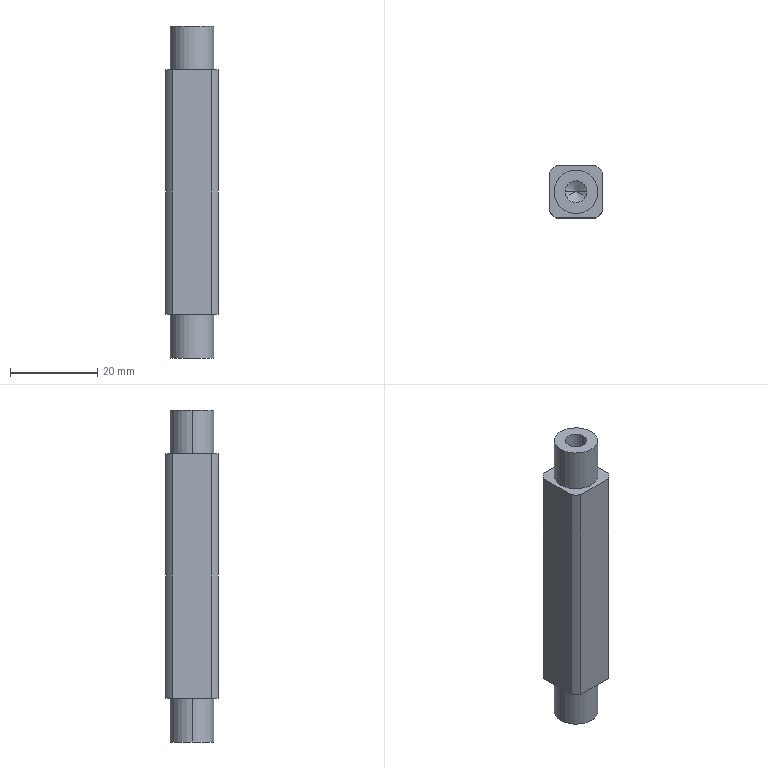Part | STEP file | Fixed shaft QY-1-07 | 1 solid | 20 faces | box 12 x 12 x 76 mm | volume 9102 mm3 | cylinder 10 | plane 8 | cone 2 | commonest cylinder face diameters 10 x4 15 x4 5 x2
STEP:
#1=CARTESIAN_POINT('',(0.,0.,0.));
#2=DIRECTION('',(0.,0.,1.));
#3=DIRECTION('',(1.,0.,0.));
#4=AXIS2_PLACEMENT_3D('',#1,#2,#3);
#5=CARTESIAN_POINT('',(2.5,0.,23.));
#6=VERTEX_POINT('',#5);
#7=CARTESIAN_POINT('',(2.5,0.,38.));
#8=VERTEX_POINT('',#7);
#9=CARTESIAN_POINT('',(2.5,0.,38.));
#10=DIRECTION('',(0.,0.,1.));
#11=VECTOR('',#10,1.);
#12=LINE('',#9,#11);
#13=CARTESIAN_POINT('',(0.,0.,38.));
#14=DIRECTION('',(0.,0.,1.));
#15=DIRECTION('',(1.,0.,0.));
#16=AXIS2_PLACEMENT_3D('',#13,#14,#15);
#17=CYLINDRICAL_SURFACE('',#16,2.5);
#18=CARTESIAN_POINT('',(6.283,0.));
#19=DIRECTION('',(0.,1.));
#20=VECTOR('',#19,1.);
#21=LINE('',#18,#20);
#22=(GEOMETRIC_REPRESENTATION_CONTEXT(2)PARAMETRIC_REPRESENTATION_CONTEXT()REPRESENTATION_CONTEXT('',''));
#23=DEFINITIONAL_REPRESENTATION('',(#21),#22);
#24=PCURVE('',#17,#23);
#25=CARTESIAN_POINT('',(0.,0.,38.));
#26=DIRECTION('',(0.,0.,1.));
#27=DIRECTION('',(1.,0.,0.));
#28=AXIS2_PLACEMENT_3D('',#25,#26,#27);
#29=CYLINDRICAL_SURFACE('',#28,2.5);
#30=CARTESIAN_POINT('',(0.,0.));
#31=DIRECTION('',(0.,1.));
#32=VECTOR('',#31,1.);
#33=LINE('',#30,#32);
#34=(GEOMETRIC_REPRESENTATION_CONTEXT(2)PARAMETRIC_REPRESENTATION_CONTEXT()REPRESENTATION_CONTEXT('',''));
#35=DEFINITIONAL_REPRESENTATION('',(#33),#34);
#36=PCURVE('',#29,#35);
#37=SURFACE_CURVE('',#12,(#24,#36),.PCURVE_S1.);
#38=EDGE_CURVE('',#6,#8,#37,.T.);
#39=ORIENTED_EDGE('',*,*,#38,.T.);
#40=CARTESIAN_POINT('',(-2.5,0.,38.));
#41=VERTEX_POINT('',#40);
#42=CARTESIAN_POINT('',(0.,0.,38.));
#43=DIRECTION('',(0.,0.,1.));
#44=DIRECTION('',(1.,0.,0.));
#45=AXIS2_PLACEMENT_3D('',#42,#43,#44);
#46=CIRCLE('',#45,2.5);
#47=CARTESIAN_POINT('',(0.,0.));
#48=DIRECTION('',(1.,0.));
#49=VECTOR('',#48,1.);
#50=LINE('',#47,#49);
#51=(GEOMETRIC_REPRESENTATION_CONTEXT(2)PARAMETRIC_REPRESENTATION_CONTEXT()REPRESENTATION_CONTEXT('',''));
#52=DEFINITIONAL_REPRESENTATION('',(#50),#51);
#53=PCURVE('',#17,#52);
#54=CARTESIAN_POINT('',(0.,0.,38.));
#55=DIRECTION('',(0.,0.,1.));
#56=DIRECTION('',(1.,0.,0.));
#57=AXIS2_PLACEMENT_3D('',#54,#55,#56);
#58=PLANE('',#57);
#59=CARTESIAN_POINT('',(0.,0.));
#60=DIRECTION('',(1.,0.));
#61=AXIS2_PLACEMENT_2D('',#59,#60);
#62=CIRCLE('',#61,2.5);
#63=(GEOMETRIC_REPRESENTATION_CONTEXT(2)PARAMETRIC_REPRESENTATION_CONTEXT()REPRESENTATION_CONTEXT('',''));
#64=DEFINITIONAL_REPRESENTATION('',(#62),#63);
#65=PCURVE('',#58,#64);
#66=SURFACE_CURVE('',#46,(#53,#65),.PCURVE_S1.);
#67=EDGE_CURVE('',#41,#8,#66,.T.);
#68=ORIENTED_EDGE('',*,*,#67,.F.);
#69=CARTESIAN_POINT('',(-2.5,0.,23.));
#70=VERTEX_POINT('',#69);
#71=CARTESIAN_POINT('',(-2.5,0.,38.));
#72=DIRECTION('',(0.,0.,1.));
#73=VECTOR('',#72,1.);
#74=LINE('',#71,#73);
#75=CARTESIAN_POINT('',(3.142,0.));
#76=DIRECTION('',(0.,1.));
#77=VECTOR('',#76,1.);
#78=LINE('',#75,#77);
#79=(GEOMETRIC_REPRESENTATION_CONTEXT(2)PARAMETRIC_REPRESENTATION_CONTEXT()REPRESENTATION_CONTEXT('',''));
#80=DEFINITIONAL_REPRESENTATION('',(#78),#79);
#81=PCURVE('',#17,#80);
#82=CARTESIAN_POINT('',(3.142,0.));
#83=DIRECTION('',(0.,1.));
#84=VECTOR('',#83,1.);
#85=LINE('',#82,#84);
#86=(GEOMETRIC_REPRESENTATION_CONTEXT(2)PARAMETRIC_REPRESENTATION_CONTEXT()REPRESENTATION_CONTEXT('',''));
#87=DEFINITIONAL_REPRESENTATION('',(#85),#86);
#88=PCURVE('',#29,#87);
#89=SURFACE_CURVE('',#74,(#81,#88),.PCURVE_S1.);
#90=EDGE_CURVE('',#70,#41,#89,.T.);
#91=ORIENTED_EDGE('',*,*,#90,.F.);
#92=CARTESIAN_POINT('',(0.,0.,23.));
#93=DIRECTION('',(0.,0.,1.));
#94=DIRECTION('',(1.,0.,0.));
#95=AXIS2_PLACEMENT_3D('',#92,#93,#94);
#96=CIRCLE('',#95,2.5);
#97=CARTESIAN_POINT('',(0.,-15.));
#98=DIRECTION('',(1.,0.));
#99=VECTOR('',#98,1.);
#100=LINE('',#97,#99);
#101=(GEOMETRIC_REPRESENTATION_CONTEXT(2)PARAMETRIC_REPRESENTATION_CONTEXT()REPRESENTATION_CONTEXT('',''));
#102=DEFINITIONAL_REPRESENTATION('',(#100),#101);
#103=PCURVE('',#17,#102);
#104=CARTESIAN_POINT('',(0.,0.,23.));
#105=DIRECTION('',(0.,0.,1.));
#106=DIRECTION('',(1.,0.,0.));
#107=AXIS2_PLACEMENT_3D('',#104,#105,#106);
#108=CONICAL_SURFACE('',#107,2.5,1.03);
#109=CARTESIAN_POINT('',(0.,0.));
#110=DIRECTION('',(1.,0.));
#111=VECTOR('',#110,1.);
#112=LINE('',#109,#111);
#113=(GEOMETRIC_REPRESENTATION_CONTEXT(2)PARAMETRIC_REPRESENTATION_CONTEXT()REPRESENTATION_CONTEXT('',''));
#114=DEFINITIONAL_REPRESENTATION('',(#112),#113);
#115=PCURVE('',#108,#114);
#116=SURFACE_CURVE('',#96,(#103,#115),.PCURVE_S1.);
#117=EDGE_CURVE('',#70,#6,#116,.T.);
#118=ORIENTED_EDGE('',*,*,#117,.T.);
#119=EDGE_LOOP('',(#39,#68,#91,#118));
#120=FACE_BOUND('',#119,.F.);
#121=ADVANCED_FACE('',(#120),#17,.F.);
#122=ORIENTED_EDGE('',*,*,#117,.F.);
#123=CARTESIAN_POINT('',(0.,0.,21.498));
#124=VERTEX_POINT('',#123);
#125=CARTESIAN_POINT('',(-2.5,0.,23.));
#126=DIRECTION('',(-0.8572,0.,0.515));
#127=VECTOR('',#126,1.);
#128=LINE('',#125,#127);
#129=CARTESIAN_POINT('',(3.142,0.));
#130=DIRECTION('',(0.,1.));
#131=VECTOR('',#130,1.);
#132=LINE('',#129,#131);
#133=(GEOMETRIC_REPRESENTATION_CONTEXT(2)PARAMETRIC_REPRESENTATION_CONTEXT()REPRESENTATION_CONTEXT('',''));
#134=DEFINITIONAL_REPRESENTATION('',(#132),#133);
#135=PCURVE('',#108,#134);
#136=CARTESIAN_POINT('',(0.,0.,23.));
#137=DIRECTION('',(0.,0.,1.));
#138=DIRECTION('',(1.,0.,0.));
#139=AXIS2_PLACEMENT_3D('',#136,#137,#138);
#140=CONICAL_SURFACE('',#139,2.5,1.03);
#141=CARTESIAN_POINT('',(3.142,0.));
#142=DIRECTION('',(0.,1.));
#143=VECTOR('',#142,1.);
#144=LINE('',#141,#143);
#145=(GEOMETRIC_REPRESENTATION_CONTEXT(2)PARAMETRIC_REPRESENTATION_CONTEXT()REPRESENTATION_CONTEXT('',''));
#146=DEFINITIONAL_REPRESENTATION('',(#144),#145);
#147=PCURVE('',#140,#146);
#148=SURFACE_CURVE('',#128,(#135,#147),.PCURVE_S1.);
#149=EDGE_CURVE('',#124,#70,#148,.T.);
#150=ORIENTED_EDGE('',*,*,#149,.F.);
#151=CARTESIAN_POINT('',(2.5,0.,23.));
#152=DIRECTION('',(0.8572,0.,0.515));
#153=VECTOR('',#152,1.);
#154=LINE('',#151,#153);
#155=CARTESIAN_POINT('',(6.283,0.));
#156=DIRECTION('',(0.,1.));
#157=VECTOR('',#156,1.);
#158=LINE('',#155,#157);
#159=(GEOMETRIC_REPRESENTATION_CONTEXT(2)PARAMETRIC_REPRESENTATION_CONTEXT()REPRESENTATION_CONTEXT('',''));
#160=DEFINITIONAL_REPRESENTATION('',(#158),#159);
#161=PCURVE('',#108,#160);
#162=CARTESIAN_POINT('',(0.,0.));
#163=DIRECTION('',(0.,1.));
#164=VECTOR('',#163,1.);
#165=LINE('',#162,#164);
#166=(GEOMETRIC_REPRESENTATION_CONTEXT(2)PARAMETRIC_REPRESENTATION_CONTEXT()REPRESENTATION_CONTEXT('',''));
#167=DEFINITIONAL_REPRESENTATION('',(#165),#166);
#168=PCURVE('',#140,#167);
#169=SURFACE_CURVE('',#154,(#161,#168),.PCURVE_S1.);
#170=EDGE_CURVE('',#124,#6,#169,.T.);
#171=ORIENTED_EDGE('',*,*,#170,.T.);
#172=EDGE_LOOP('',(#122,#150,#171));
#173=FACE_BOUND('',#172,.F.);
#174=ADVANCED_FACE('',(#173),#108,.F.);
#175=CARTESIAN_POINT('',(5.,0.,-38.));
#176=VERTEX_POINT('',#175);
#177=CARTESIAN_POINT('',(-5.,0.,-38.));
#178=VERTEX_POINT('',#177);
#179=CARTESIAN_POINT('',(0.,0.,-38.));
#180=DIRECTION('',(0.,0.,1.));
#181=DIRECTION('',(1.,0.,0.));
#182=AXIS2_PLACEMENT_3D('',#179,#180,#181);
#183=CIRCLE('',#182,5.);
#184=CARTESIAN_POINT('',(0.,0.,-38.));
#185=DIRECTION('',(0.,0.,1.));
#186=DIRECTION('',(1.,0.,0.));
#187=AXIS2_PLACEMENT_3D('',#184,#185,#186);
#188=CYLINDRICAL_SURFACE('',#187,5.);
#189=CARTESIAN_POINT('',(0.,0.));
#190=DIRECTION('',(1.,0.));
#191=VECTOR('',#190,1.);
#192=LINE('',#189,#191);
#193=(GEOMETRIC_REPRESENTATION_CONTEXT(2)PARAMETRIC_REPRESENTATION_CONTEXT()REPRESENTATION_CONTEXT('',''));
#194=DEFINITIONAL_REPRESENTATION('',(#192),#193);
#195=PCURVE('',#188,#194);
#196=CARTESIAN_POINT('',(0.,0.,-38.));
#197=DIRECTION('',(0.,0.,-1.));
#198=DIRECTION('',(1.,0.,0.));
#199=AXIS2_PLACEMENT_3D('',#196,#197,#198);
#200=PLANE('',#199);
#201=CARTESIAN_POINT('',(5.,0.));
#202=CARTESIAN_POINT('',(5.,-8.66));
#203=CARTESIAN_POINT('',(-2.5,-4.33));
#204=CARTESIAN_POINT('',(-10.,0.));
#205=CARTESIAN_POINT('',(-2.5,4.33));
#206=CARTESIAN_POINT('',(5.,8.66));
#207=CARTESIAN_POINT('',(5.,0.));
#208=(BOUNDED_CURVE()B_SPLINE_CURVE(2,(#201,#202,#203,#204,#205,#206,#207),.UNSPECIFIED.,.T.,.F.)B_SPLINE_CURVE_WITH_KNOTS((1,2,2,2,2,1),(-2.094,0.,2.094,4.189,6.283,8.378),.UNSPECIFIED.)CURVE()GEOMETRIC_REPRESENTATION_ITEM()RATIONAL_B_SPLINE_CURVE((1.,0.5,1.,0.5,1.,0.5,1.))REPRESENTATION_ITEM(''));
#209=(GEOMETRIC_REPRESENTATION_CONTEXT(2)PARAMETRIC_REPRESENTATION_CONTEXT()REPRESENTATION_CONTEXT('',''));
#210=DEFINITIONAL_REPRESENTATION('',(#208),#209);
#211=PCURVE('',#200,#210);
#212=SURFACE_CURVE('',#183,(#195,#211),.PCURVE_S1.);
#213=EDGE_CURVE('',#176,#178,#212,.T.);
#214=ORIENTED_EDGE('',*,*,#213,.T.);
#215=CARTESIAN_POINT('',(-5.,0.,-28.));
#216=VERTEX_POINT('',#215);
#217=CARTESIAN_POINT('',(-5.,0.,-38.));
#218=DIRECTION('',(0.,0.,1.));
#219=VECTOR('',#218,1.);
#220=LINE('',#217,#219);
#221=CARTESIAN_POINT('',(3.142,0.));
#222=DIRECTION('',(0.,1.));
#223=VECTOR('',#222,1.);
#224=LINE('',#221,#223);
#225=(GEOMETRIC_REPRESENTATION_CONTEXT(2)PARAMETRIC_REPRESENTATION_CONTEXT()REPRESENTATION_CONTEXT('',''));
#226=DEFINITIONAL_REPRESENTATION('',(#224),#225);
#227=PCURVE('',#188,#226);
#228=CARTESIAN_POINT('',(0.,0.,-38.));
#229=DIRECTION('',(0.,0.,1.));
#230=DIRECTION('',(1.,0.,0.));
#231=AXIS2_PLACEMENT_3D('',#228,#229,#230);
#232=CYLINDRICAL_SURFACE('',#231,5.);
#233=CARTESIAN_POINT('',(3.142,0.));
#234=DIRECTION('',(0.,1.));
#235=VECTOR('',#234,1.);
#236=LINE('',#233,#235);
#237=(GEOMETRIC_REPRESENTATION_CONTEXT(2)PARAMETRIC_REPRESENTATION_CONTEXT()REPRESENTATION_CONTEXT('',''));
#238=DEFINITIONAL_REPRESENTATION('',(#236),#237);
#239=PCURVE('',#232,#238);
#240=SURFACE_CURVE('',#220,(#227,#239),.PCURVE_S1.);
#241=EDGE_CURVE('',#178,#216,#240,.T.);
#242=ORIENTED_EDGE('',*,*,#241,.T.);
#243=CARTESIAN_POINT('',(5.,0.,-28.));
#244=VERTEX_POINT('',#243);
#245=CARTESIAN_POINT('',(0.,0.,-28.));
#246=DIRECTION('',(0.,0.,1.));
#247=DIRECTION('',(1.,0.,0.));
#248=AXIS2_PLACEMENT_3D('',#245,#246,#247);
#249=CIRCLE('',#248,5.);
#250=CARTESIAN_POINT('',(0.,10.));
#251=DIRECTION('',(1.,0.));
#252=VECTOR('',#251,1.);
#253=LINE('',#250,#252);
#254=(GEOMETRIC_REPRESENTATION_CONTEXT(2)PARAMETRIC_REPRESENTATION_CONTEXT()REPRESENTATION_CONTEXT('',''));
#255=DEFINITIONAL_REPRESENTATION('',(#253),#254);
#256=PCURVE('',#188,#255);
#257=CARTESIAN_POINT('',(0.,0.,-28.));
#258=DIRECTION('',(0.,0.,1.));
#259=DIRECTION('',(1.,0.,0.));
#260=AXIS2_PLACEMENT_3D('',#257,#258,#259);
#261=PLANE('',#260);
#262=CARTESIAN_POINT('',(0.,0.));
#263=DIRECTION('',(1.,0.));
#264=AXIS2_PLACEMENT_2D('',#262,#263);
#265=CIRCLE('',#264,5.);
#266=(GEOMETRIC_REPRESENTATION_CONTEXT(2)PARAMETRIC_REPRESENTATION_CONTEXT()REPRESENTATION_CONTEXT('',''));
#267=DEFINITIONAL_REPRESENTATION('',(#265),#266);
#268=PCURVE('',#261,#267);
#269=SURFACE_CURVE('',#249,(#256,#268),.PCURVE_S1.);
#270=EDGE_CURVE('',#244,#216,#269,.T.);
#271=ORIENTED_EDGE('',*,*,#270,.F.);
#272=CARTESIAN_POINT('',(5.,0.,-38.));
#273=DIRECTION('',(0.,0.,1.));
#274=VECTOR('',#273,1.);
#275=LINE('',#272,#274);
#276=CARTESIAN_POINT('',(0.,0.));
#277=DIRECTION('',(0.,1.));
#278=VECTOR('',#277,1.);
#279=LINE('',#276,#278);
#280=(GEOMETRIC_REPRESENTATION_CONTEXT(2)PARAMETRIC_REPRESENTATION_CONTEXT()REPRESENTATION_CONTEXT('',''));
#281=DEFINITIONAL_REPRESENTATION('',(#279),#280);
#282=PCURVE('',#188,#281);
#283=CARTESIAN_POINT('',(6.283,0.));
#284=DIRECTION('',(0.,1.));
#285=VECTOR('',#284,1.);
#286=LINE('',#283,#285);
#287=(GEOMETRIC_REPRESENTATION_CONTEXT(2)PARAMETRIC_REPRESENTATION_CONTEXT()REPRESENTATION_CONTEXT('',''));
#288=DEFINITIONAL_REPRESENTATION('',(#286),#287);
#289=PCURVE('',#232,#288);
#290=SURFACE_CURVE('',#275,(#282,#289),.PCURVE_S1.);
#291=EDGE_CURVE('',#176,#244,#290,.T.);
#292=ORIENTED_EDGE('',*,*,#291,.F.);
#293=EDGE_LOOP('',(#214,#242,#271,#292));
#294=FACE_BOUND('',#293,.T.);
#295=ADVANCED_FACE('',(#294),#188,.T.);
#296=CARTESIAN_POINT('',(5.,0.,38.));
#297=VERTEX_POINT('',#296);
#298=CARTESIAN_POINT('',(-5.,0.,38.));
#299=VERTEX_POINT('',#298);
#300=CARTESIAN_POINT('',(0.,0.,38.));
#301=DIRECTION('',(0.,0.,1.));
#302=DIRECTION('',(1.,0.,0.));
#303=AXIS2_PLACEMENT_3D('',#300,#301,#302);
#304=CIRCLE('',#303,5.);
#305=CARTESIAN_POINT('',(0.,0.,38.));
#306=DIRECTION('',(0.,0.,-1.));
#307=DIRECTION('',(-1.,0.,0.));
#308=AXIS2_PLACEMENT_3D('',#305,#306,#307);
#309=CYLINDRICAL_SURFACE('',#308,5.);
#310=CARTESIAN_POINT('',(3.142,0.));
#311=DIRECTION('',(-1.,0.));
#312=VECTOR('',#311,1.);
#313=LINE('',#310,#312);
#314=(GEOMETRIC_REPRESENTATION_CONTEXT(2)PARAMETRIC_REPRESENTATION_CONTEXT()REPRESENTATION_CONTEXT('',''));
#315=DEFINITIONAL_REPRESENTATION('',(#313),#314);
#316=PCURVE('',#309,#315);
#317=CARTESIAN_POINT('',(0.,0.));
#318=DIRECTION('',(1.,0.));
#319=AXIS2_PLACEMENT_2D('',#317,#318);
#320=CIRCLE('',#319,5.);
#321=(GEOMETRIC_REPRESENTATION_CONTEXT(2)PARAMETRIC_REPRESENTATION_CONTEXT()REPRESENTATION_CONTEXT('',''));
#322=DEFINITIONAL_REPRESENTATION('',(#320),#321);
#323=PCURVE('',#58,#322);
#324=SURFACE_CURVE('',#304,(#316,#323),.PCURVE_S1.);
#325=EDGE_CURVE('',#297,#299,#324,.T.);
#326=ORIENTED_EDGE('',*,*,#325,.F.);
#327=CARTESIAN_POINT('',(5.,0.,28.));
#328=VERTEX_POINT('',#327);
#329=CARTESIAN_POINT('',(5.,0.,38.));
#330=DIRECTION('',(0.,0.,-1.));
#331=VECTOR('',#330,1.);
#332=LINE('',#329,#331);
#333=CARTESIAN_POINT('',(3.142,0.));
#334=DIRECTION('',(0.,1.));
#335=VECTOR('',#334,1.);
#336=LINE('',#333,#335);
#337=(GEOMETRIC_REPRESENTATION_CONTEXT(2)PARAMETRIC_REPRESENTATION_CONTEXT()REPRESENTATION_CONTEXT('',''));
#338=DEFINITIONAL_REPRESENTATION('',(#336),#337);
#339=PCURVE('',#309,#338);
#340=CARTESIAN_POINT('',(0.,0.,38.));
#341=DIRECTION('',(0.,0.,-1.));
#342=DIRECTION('',(-1.,0.,0.));
#343=AXIS2_PLACEMENT_3D('',#340,#341,#342);
#344=CYLINDRICAL_SURFACE('',#343,5.);
#345=CARTESIAN_POINT('',(3.142,0.));
#346=DIRECTION('',(0.,1.));
#347=VECTOR('',#346,1.);
#348=LINE('',#345,#347);
#349=(GEOMETRIC_REPRESENTATION_CONTEXT(2)PARAMETRIC_REPRESENTATION_CONTEXT()REPRESENTATION_CONTEXT('',''));
#350=DEFINITIONAL_REPRESENTATION('',(#348),#349);
#351=PCURVE('',#344,#350);
#352=SURFACE_CURVE('',#332,(#339,#351),.PCURVE_S1.);
#353=EDGE_CURVE('',#297,#328,#352,.T.);
#354=ORIENTED_EDGE('',*,*,#353,.T.);
#355=CARTESIAN_POINT('',(-5.,0.,28.));
#356=VERTEX_POINT('',#355);
#357=CARTESIAN_POINT('',(0.,0.,28.));
#358=DIRECTION('',(0.,0.,1.));
#359=DIRECTION('',(1.,0.,0.));
#360=AXIS2_PLACEMENT_3D('',#357,#358,#359);
#361=CIRCLE('',#360,5.);
#362=CARTESIAN_POINT('',(3.142,10.));
#363=DIRECTION('',(-1.,0.));
#364=VECTOR('',#363,1.);
#365=LINE('',#362,#364);
#366=(GEOMETRIC_REPRESENTATION_CONTEXT(2)PARAMETRIC_REPRESENTATION_CONTEXT()REPRESENTATION_CONTEXT('',''));
#367=DEFINITIONAL_REPRESENTATION('',(#365),#366);
#368=PCURVE('',#309,#367);
#369=CARTESIAN_POINT('',(0.,0.,28.));
#370=DIRECTION('',(0.,0.,1.));
#371=DIRECTION('',(1.,0.,0.));
#372=AXIS2_PLACEMENT_3D('',#369,#370,#371);
#373=PLANE('',#372);
#374=CARTESIAN_POINT('',(0.,0.));
#375=DIRECTION('',(1.,0.));
#376=AXIS2_PLACEMENT_2D('',#374,#375);
#377=CIRCLE('',#376,5.);
#378=(GEOMETRIC_REPRESENTATION_CONTEXT(2)PARAMETRIC_REPRESENTATION_CONTEXT()REPRESENTATION_CONTEXT('',''));
#379=DEFINITIONAL_REPRESENTATION('',(#377),#378);
#380=PCURVE('',#373,#379);
#381=SURFACE_CURVE('',#361,(#368,#380),.PCURVE_S1.);
#382=EDGE_CURVE('',#328,#356,#381,.T.);
#383=ORIENTED_EDGE('',*,*,#382,.T.);
#384=CARTESIAN_POINT('',(-5.,0.,38.));
#385=DIRECTION('',(0.,0.,-1.));
#386=VECTOR('',#385,1.);
#387=LINE('',#384,#386);
#388=CARTESIAN_POINT('',(0.,0.));
#389=DIRECTION('',(0.,1.));
#390=VECTOR('',#389,1.);
#391=LINE('',#388,#390);
#392=(GEOMETRIC_REPRESENTATION_CONTEXT(2)PARAMETRIC_REPRESENTATION_CONTEXT()REPRESENTATION_CONTEXT('',''));
#393=DEFINITIONAL_REPRESENTATION('',(#391),#392);
#394=PCURVE('',#309,#393);
#395=CARTESIAN_POINT('',(6.283,0.));
#396=DIRECTION('',(0.,1.));
#397=VECTOR('',#396,1.);
#398=LINE('',#395,#397);
#399=(GEOMETRIC_REPRESENTATION_CONTEXT(2)PARAMETRIC_REPRESENTATION_CONTEXT()REPRESENTATION_CONTEXT('',''));
#400=DEFINITIONAL_REPRESENTATION('',(#398),#399);
#401=PCURVE('',#344,#400);
#402=SURFACE_CURVE('',#387,(#394,#401),.PCURVE_S1.);
#403=EDGE_CURVE('',#299,#356,#402,.T.);
#404=ORIENTED_EDGE('',*,*,#403,.F.);
#405=EDGE_LOOP('',(#326,#354,#383,#404));
#406=FACE_BOUND('',#405,.T.);
#407=ADVANCED_FACE('',(#406),#309,.T.);
#408=CARTESIAN_POINT('',(-6.,-4.5,-28.));
#409=VERTEX_POINT('',#408);
#410=CARTESIAN_POINT('',(-4.5,-6.,-28.));
#411=VERTEX_POINT('',#410);
#412=CARTESIAN_POINT('',(0.,0.,-28.));
#413=DIRECTION('',(0.,0.,1.));
#414=DIRECTION('',(1.,0.,0.));
#415=AXIS2_PLACEMENT_3D('',#412,#413,#414);
#416=CIRCLE('',#415,7.5);
#417=CARTESIAN_POINT('',(0.,0.,28.));
#418=DIRECTION('',(0.,0.,-1.));
#419=DIRECTION('',(-1.,0.,0.));
#420=AXIS2_PLACEMENT_3D('',#417,#418,#419);
#421=CYLINDRICAL_SURFACE('',#420,7.5);
#422=CARTESIAN_POINT('',(9.425,56.));
#423=DIRECTION('',(-1.,0.));
#424=VECTOR('',#423,1.);
#425=LINE('',#422,#424);
#426=(GEOMETRIC_REPRESENTATION_CONTEXT(2)PARAMETRIC_REPRESENTATION_CONTEXT()REPRESENTATION_CONTEXT('',''));
#427=DEFINITIONAL_REPRESENTATION('',(#425),#426);
#428=PCURVE('',#421,#427);
#429=CARTESIAN_POINT('',(0.,0.));
#430=DIRECTION('',(1.,0.));
#431=AXIS2_PLACEMENT_2D('',#429,#430);
#432=CIRCLE('',#431,7.5);
#433=(GEOMETRIC_REPRESENTATION_CONTEXT(2)PARAMETRIC_REPRESENTATION_CONTEXT()REPRESENTATION_CONTEXT('',''));
#434=DEFINITIONAL_REPRESENTATION('',(#432),#433);
#435=PCURVE('',#261,#434);
#436=SURFACE_CURVE('',#416,(#428,#435),.PCURVE_S1.);
#437=EDGE_CURVE('',#409,#411,#436,.T.);
#438=ORIENTED_EDGE('',*,*,#437,.T.);
#439=CARTESIAN_POINT('',(-4.5,-6.,28.));
#440=VERTEX_POINT('',#439);
#441=CARTESIAN_POINT('',(-4.5,-6.,28.));
#442=DIRECTION('',(0.,0.,-1.));
#443=VECTOR('',#442,1.);
#444=LINE('',#441,#443);
#445=CARTESIAN_POINT('',(5.356,0.));
#446=DIRECTION('',(0.,1.));
#447=VECTOR('',#446,1.);
#448=LINE('',#445,#447);
#449=(GEOMETRIC_REPRESENTATION_CONTEXT(2)PARAMETRIC_REPRESENTATION_CONTEXT()REPRESENTATION_CONTEXT('',''));
#450=DEFINITIONAL_REPRESENTATION('',(#448),#449);
#451=PCURVE('',#421,#450);
#452=CARTESIAN_POINT('',(-4.5,-6.,28.));
#453=DIRECTION('',(0.,1.,0.));
#454=DIRECTION('',(0.,0.,1.));
#455=AXIS2_PLACEMENT_3D('',#452,#453,#454);
#456=PLANE('',#455);
#457=CARTESIAN_POINT('',(0.,0.));
#458=DIRECTION('',(-1.,0.));
#459=VECTOR('',#458,1.);
#460=LINE('',#457,#459);
#461=(GEOMETRIC_REPRESENTATION_CONTEXT(2)PARAMETRIC_REPRESENTATION_CONTEXT()REPRESENTATION_CONTEXT('',''));
#462=DEFINITIONAL_REPRESENTATION('',(#460),#461);
#463=PCURVE('',#456,#462);
#464=SURFACE_CURVE('',#444,(#451,#463),.PCURVE_S1.);
#465=EDGE_CURVE('',#440,#411,#464,.T.);
#466=ORIENTED_EDGE('',*,*,#465,.F.);
#467=CARTESIAN_POINT('',(-6.,-4.5,28.));
#468=VERTEX_POINT('',#467);
#469=CARTESIAN_POINT('',(0.,0.,28.));
#470=DIRECTION('',(0.,0.,1.));
#471=DIRECTION('',(1.,0.,0.));
#472=AXIS2_PLACEMENT_3D('',#469,#470,#471);
#473=CIRCLE('',#472,7.5);
#474=CARTESIAN_POINT('',(9.425,0.));
#475=DIRECTION('',(-1.,0.));
#476=VECTOR('',#475,1.);
#477=LINE('',#474,#476);
#478=(GEOMETRIC_REPRESENTATION_CONTEXT(2)PARAMETRIC_REPRESENTATION_CONTEXT()REPRESENTATION_CONTEXT('',''));
#479=DEFINITIONAL_REPRESENTATION('',(#477),#478);
#480=PCURVE('',#421,#479);
#481=CARTESIAN_POINT('',(0.,0.));
#482=DIRECTION('',(1.,0.));
#483=AXIS2_PLACEMENT_2D('',#481,#482);
#484=CIRCLE('',#483,7.5);
#485=(GEOMETRIC_REPRESENTATION_CONTEXT(2)PARAMETRIC_REPRESENTATION_CONTEXT()REPRESENTATION_CONTEXT('',''));
#486=DEFINITIONAL_REPRESENTATION('',(#484),#485);
#487=PCURVE('',#373,#486);
#488=SURFACE_CURVE('',#473,(#480,#487),.PCURVE_S1.);
#489=EDGE_CURVE('',#468,#440,#488,.T.);
#490=ORIENTED_EDGE('',*,*,#489,.F.);
#491=CARTESIAN_POINT('',(-6.,-4.5,28.));
#492=DIRECTION('',(0.,0.,-1.));
#493=VECTOR('',#492,1.);
#494=LINE('',#491,#493);
#495=CARTESIAN_POINT('',(5.64,0.));
#496=DIRECTION('',(0.,1.));
#497=VECTOR('',#496,1.);
#498=LINE('',#495,#497);
#499=(GEOMETRIC_REPRESENTATION_CONTEXT(2)PARAMETRIC_REPRESENTATION_CONTEXT()REPRESENTATION_CONTEXT('',''));
#500=DEFINITIONAL_REPRESENTATION('',(#498),#499);
#501=PCURVE('',#421,#500);
#502=CARTESIAN_POINT('',(-6.,4.5,28.));
#503=DIRECTION('',(1.,0.,0.));
#504=DIRECTION('',(0.,1.,0.));
#505=AXIS2_PLACEMENT_3D('',#502,#503,#504);
#506=PLANE('',#505);
#507=CARTESIAN_POINT('',(-9.,0.));
#508=DIRECTION('',(0.,-1.));
#509=VECTOR('',#508,1.);
#510=LINE('',#507,#509);
#511=(GEOMETRIC_REPRESENTATION_CONTEXT(2)PARAMETRIC_REPRESENTATION_CONTEXT()REPRESENTATION_CONTEXT('',''));
#512=DEFINITIONAL_REPRESENTATION('',(#510),#511);
#513=PCURVE('',#506,#512);
#514=SURFACE_CURVE('',#494,(#501,#513),.PCURVE_S1.);
#515=EDGE_CURVE('',#468,#409,#514,.T.);
#516=ORIENTED_EDGE('',*,*,#515,.T.);
#517=EDGE_LOOP('',(#438,#466,#490,#516));
#518=FACE_BOUND('',#517,.T.);
#519=ADVANCED_FACE('',(#518),#421,.T.);
#520=CARTESIAN_POINT('',(4.5,-6.,-28.));
#521=VERTEX_POINT('',#520);
#522=CARTESIAN_POINT('',(-4.5,-6.,-28.));
#523=DIRECTION('',(1.,0.,0.));
#524=VECTOR('',#523,1.);
#525=LINE('',#522,#524);
#526=CARTESIAN_POINT('',(-56.,0.));
#527=DIRECTION('',(0.,1.));
#528=VECTOR('',#527,1.);
#529=LINE('',#526,#528);
#530=(GEOMETRIC_REPRESENTATION_CONTEXT(2)PARAMETRIC_REPRESENTATION_CONTEXT()REPRESENTATION_CONTEXT('',''));
#531=DEFINITIONAL_REPRESENTATION('',(#529),#530);
#532=PCURVE('',#456,#531);
#533=CARTESIAN_POINT('',(-4.5,-6.));
#534=DIRECTION('',(1.,0.));
#535=VECTOR('',#534,1.);
#536=LINE('',#533,#535);
#537=(GEOMETRIC_REPRESENTATION_CONTEXT(2)PARAMETRIC_REPRESENTATION_CONTEXT()REPRESENTATION_CONTEXT('',''));
#538=DEFINITIONAL_REPRESENTATION('',(#536),#537);
#539=PCURVE('',#261,#538);
#540=SURFACE_CURVE('',#525,(#532,#539),.PCURVE_S1.);
#541=EDGE_CURVE('',#411,#521,#540,.T.);
#542=ORIENTED_EDGE('',*,*,#541,.T.);
#543=CARTESIAN_POINT('',(4.5,-6.,28.));
#544=VERTEX_POINT('',#543);
#545=CARTESIAN_POINT('',(4.5,-6.,28.));
#546=DIRECTION('',(0.,0.,-1.));
#547=VECTOR('',#546,1.);
#548=LINE('',#545,#547);
#549=CARTESIAN_POINT('',(0.,9.));
#550=DIRECTION('',(-1.,0.));
#551=VECTOR('',#550,1.);
#552=LINE('',#549,#551);
#553=(GEOMETRIC_REPRESENTATION_CONTEXT(2)PARAMETRIC_REPRESENTATION_CONTEXT()REPRESENTATION_CONTEXT('',''));
#554=DEFINITIONAL_REPRESENTATION('',(#552),#553);
#555=PCURVE('',#456,#554);
#556=CARTESIAN_POINT('',(0.,0.,28.));
#557=DIRECTION('',(0.,0.,-1.));
#558=DIRECTION('',(-1.,0.,0.));
#559=AXIS2_PLACEMENT_3D('',#556,#557,#558);
#560=CYLINDRICAL_SURFACE('',#559,7.5);
#561=CARTESIAN_POINT('',(4.069,0.));
#562=DIRECTION('',(0.,1.));
#563=VECTOR('',#562,1.);
#564=LINE('',#561,#563);
#565=(GEOMETRIC_REPRESENTATION_CONTEXT(2)PARAMETRIC_REPRESENTATION_CONTEXT()REPRESENTATION_CONTEXT('',''));
#566=DEFINITIONAL_REPRESENTATION('',(#564),#565);
#567=PCURVE('',#560,#566);
#568=SURFACE_CURVE('',#548,(#555,#567),.PCURVE_S1.);
#569=EDGE_CURVE('',#544,#521,#568,.T.);
#570=ORIENTED_EDGE('',*,*,#569,.F.);
#571=CARTESIAN_POINT('',(-4.5,-6.,28.));
#572=DIRECTION('',(1.,0.,0.));
#573=VECTOR('',#572,1.);
#574=LINE('',#571,#573);
#575=CARTESIAN_POINT('',(0.,0.));
#576=DIRECTION('',(0.,1.));
#577=VECTOR('',#576,1.);
#578=LINE('',#575,#577);
#579=(GEOMETRIC_REPRESENTATION_CONTEXT(2)PARAMETRIC_REPRESENTATION_CONTEXT()REPRESENTATION_CONTEXT('',''));
#580=DEFINITIONAL_REPRESENTATION('',(#578),#579);
#581=PCURVE('',#456,#580);
#582=CARTESIAN_POINT('',(-4.5,-6.));
#583=DIRECTION('',(1.,0.));
#584=VECTOR('',#583,1.);
#585=LINE('',#582,#584);
#586=(GEOMETRIC_REPRESENTATION_CONTEXT(2)PARAMETRIC_REPRESENTATION_CONTEXT()REPRESENTATION_CONTEXT('',''));
#587=DEFINITIONAL_REPRESENTATION('',(#585),#586);
#588=PCURVE('',#373,#587);
#589=SURFACE_CURVE('',#574,(#581,#588),.PCURVE_S1.);
#590=EDGE_CURVE('',#440,#544,#589,.T.);
#591=ORIENTED_EDGE('',*,*,#590,.F.);
#592=ORIENTED_EDGE('',*,*,#465,.T.);
#593=EDGE_LOOP('',(#542,#570,#591,#592));
#594=FACE_BOUND('',#593,.T.);
#595=ADVANCED_FACE('',(#594),#456,.F.);
#596=CARTESIAN_POINT('',(6.,-4.5,-28.));
#597=VERTEX_POINT('',#596);
#598=CARTESIAN_POINT('',(0.,0.,-28.));
#599=DIRECTION('',(0.,0.,1.));
#600=DIRECTION('',(1.,0.,0.));
#601=AXIS2_PLACEMENT_3D('',#598,#599,#600);
#602=CIRCLE('',#601,7.5);
#603=CARTESIAN_POINT('',(9.425,56.));
#604=DIRECTION('',(-1.,0.));
#605=VECTOR('',#604,1.);
#606=LINE('',#603,#605);
#607=(GEOMETRIC_REPRESENTATION_CONTEXT(2)PARAMETRIC_REPRESENTATION_CONTEXT()REPRESENTATION_CONTEXT('',''));
#608=DEFINITIONAL_REPRESENTATION('',(#606),#607);
#609=PCURVE('',#560,#608);
#610=CARTESIAN_POINT('',(0.,0.));
#611=DIRECTION('',(1.,0.));
#612=AXIS2_PLACEMENT_2D('',#610,#611);
#613=CIRCLE('',#612,7.5);
#614=(GEOMETRIC_REPRESENTATION_CONTEXT(2)PARAMETRIC_REPRESENTATION_CONTEXT()REPRESENTATION_CONTEXT('',''));
#615=DEFINITIONAL_REPRESENTATION('',(#613),#614);
#616=PCURVE('',#261,#615);
#617=SURFACE_CURVE('',#602,(#609,#616),.PCURVE_S1.);
#618=EDGE_CURVE('',#521,#597,#617,.T.);
#619=ORIENTED_EDGE('',*,*,#618,.T.);
#620=CARTESIAN_POINT('',(6.,-4.5,28.));
#621=VERTEX_POINT('',#620);
#622=CARTESIAN_POINT('',(6.,-4.5,28.));
#623=DIRECTION('',(0.,0.,-1.));
#624=VECTOR('',#623,1.);
#625=LINE('',#622,#624);
#626=CARTESIAN_POINT('',(3.785,0.));
#627=DIRECTION('',(0.,1.));
#628=VECTOR('',#627,1.);
#629=LINE('',#626,#628);
#630=(GEOMETRIC_REPRESENTATION_CONTEXT(2)PARAMETRIC_REPRESENTATION_CONTEXT()REPRESENTATION_CONTEXT('',''));
#631=DEFINITIONAL_REPRESENTATION('',(#629),#630);
#632=PCURVE('',#560,#631);
#633=CARTESIAN_POINT('',(6.,4.5,28.));
#634=DIRECTION('',(-1.,0.,0.));
#635=DIRECTION('',(0.,-1.,0.));
#636=AXIS2_PLACEMENT_3D('',#633,#634,#635);
#637=PLANE('',#636);
#638=CARTESIAN_POINT('',(9.,0.));
#639=DIRECTION('',(0.,-1.));
#640=VECTOR('',#639,1.);
#641=LINE('',#638,#640);
#642=(GEOMETRIC_REPRESENTATION_CONTEXT(2)PARAMETRIC_REPRESENTATION_CONTEXT()REPRESENTATION_CONTEXT('',''));
#643=DEFINITIONAL_REPRESENTATION('',(#641),#642);
#644=PCURVE('',#637,#643);
#645=SURFACE_CURVE('',#625,(#632,#644),.PCURVE_S1.);
#646=EDGE_CURVE('',#621,#597,#645,.T.);
#647=ORIENTED_EDGE('',*,*,#646,.F.);
#648=CARTESIAN_POINT('',(0.,0.,28.));
#649=DIRECTION('',(0.,0.,1.));
#650=DIRECTION('',(1.,0.,0.));
#651=AXIS2_PLACEMENT_3D('',#648,#649,#650);
#652=CIRCLE('',#651,7.5);
#653=CARTESIAN_POINT('',(9.425,0.));
#654=DIRECTION('',(-1.,0.));
#655=VECTOR('',#654,1.);
#656=LINE('',#653,#655);
#657=(GEOMETRIC_REPRESENTATION_CONTEXT(2)PARAMETRIC_REPRESENTATION_CONTEXT()REPRESENTATION_CONTEXT('',''));
#658=DEFINITIONAL_REPRESENTATION('',(#656),#657);
#659=PCURVE('',#560,#658);
#660=CARTESIAN_POINT('',(0.,0.));
#661=DIRECTION('',(1.,0.));
#662=AXIS2_PLACEMENT_2D('',#660,#661);
#663=CIRCLE('',#662,7.5);
#664=(GEOMETRIC_REPRESENTATION_CONTEXT(2)PARAMETRIC_REPRESENTATION_CONTEXT()REPRESENTATION_CONTEXT('',''));
#665=DEFINITIONAL_REPRESENTATION('',(#663),#664);
#666=PCURVE('',#373,#665);
#667=SURFACE_CURVE('',#652,(#659,#666),.PCURVE_S1.);
#668=EDGE_CURVE('',#544,#621,#667,.T.);
#669=ORIENTED_EDGE('',*,*,#668,.F.);
#670=ORIENTED_EDGE('',*,*,#569,.T.);
#671=EDGE_LOOP('',(#619,#647,#669,#670));
#672=FACE_BOUND('',#671,.T.);
#673=ADVANCED_FACE('',(#672),#560,.T.);
#674=CARTESIAN_POINT('',(6.,4.5,-28.));
#675=VERTEX_POINT('',#674);
#676=CARTESIAN_POINT('',(6.,4.5,-28.));
#677=DIRECTION('',(0.,1.,0.));
#678=VECTOR('',#677,1.);
#679=LINE('',#676,#678);
#680=CARTESIAN_POINT('',(0.,-56.));
#681=DIRECTION('',(-1.,0.));
#682=VECTOR('',#681,1.);
#683=LINE('',#680,#682);
#684=(GEOMETRIC_REPRESENTATION_CONTEXT(2)PARAMETRIC_REPRESENTATION_CONTEXT()REPRESENTATION_CONTEXT('',''));
#685=DEFINITIONAL_REPRESENTATION('',(#683),#684);
#686=PCURVE('',#637,#685);
#687=CARTESIAN_POINT('',(6.,4.5));
#688=DIRECTION('',(0.,1.));
#689=VECTOR('',#688,1.);
#690=LINE('',#687,#689);
#691=(GEOMETRIC_REPRESENTATION_CONTEXT(2)PARAMETRIC_REPRESENTATION_CONTEXT()REPRESENTATION_CONTEXT('',''));
#692=DEFINITIONAL_REPRESENTATION('',(#690),#691);
#693=PCURVE('',#261,#692);
#694=SURFACE_CURVE('',#679,(#686,#693),.PCURVE_S1.);
#695=EDGE_CURVE('',#597,#675,#694,.T.);
#696=ORIENTED_EDGE('',*,*,#695,.T.);
#697=CARTESIAN_POINT('',(6.,4.5,28.));
#698=VERTEX_POINT('',#697);
#699=CARTESIAN_POINT('',(6.,4.5,28.));
#700=DIRECTION('',(0.,0.,-1.));
#701=VECTOR('',#700,1.);
#702=LINE('',#699,#701);
#703=CARTESIAN_POINT('',(0.,0.));
#704=DIRECTION('',(0.,-1.));
#705=VECTOR('',#704,1.);
#706=LINE('',#703,#705);
#707=(GEOMETRIC_REPRESENTATION_CONTEXT(2)PARAMETRIC_REPRESENTATION_CONTEXT()REPRESENTATION_CONTEXT('',''));
#708=DEFINITIONAL_REPRESENTATION('',(#706),#707);
#709=PCURVE('',#637,#708);
#710=CARTESIAN_POINT('',(0.,0.,28.));
#711=DIRECTION('',(0.,0.,-1.));
#712=DIRECTION('',(-1.,0.,0.));
#713=AXIS2_PLACEMENT_3D('',#710,#711,#712);
#714=CYLINDRICAL_SURFACE('',#713,7.5);
#715=CARTESIAN_POINT('',(2.498,0.));
#716=DIRECTION('',(0.,1.));
#717=VECTOR('',#716,1.);
#718=LINE('',#715,#717);
#719=(GEOMETRIC_REPRESENTATION_CONTEXT(2)PARAMETRIC_REPRESENTATION_CONTEXT()REPRESENTATION_CONTEXT('',''));
#720=DEFINITIONAL_REPRESENTATION('',(#718),#719);
#721=PCURVE('',#714,#720);
#722=SURFACE_CURVE('',#702,(#709,#721),.PCURVE_S1.);
#723=EDGE_CURVE('',#698,#675,#722,.T.);
#724=ORIENTED_EDGE('',*,*,#723,.F.);
#725=CARTESIAN_POINT('',(6.,4.5,28.));
#726=DIRECTION('',(0.,1.,0.));
#727=VECTOR('',#726,1.);
#728=LINE('',#725,#727);
#729=CARTESIAN_POINT('',(0.,0.));
#730=DIRECTION('',(-1.,0.));
#731=VECTOR('',#730,1.);
#732=LINE('',#729,#731);
#733=(GEOMETRIC_REPRESENTATION_CONTEXT(2)PARAMETRIC_REPRESENTATION_CONTEXT()REPRESENTATION_CONTEXT('',''));
#734=DEFINITIONAL_REPRESENTATION('',(#732),#733);
#735=PCURVE('',#637,#734);
#736=CARTESIAN_POINT('',(6.,4.5));
#737=DIRECTION('',(0.,1.));
#738=VECTOR('',#737,1.);
#739=LINE('',#736,#738);
#740=(GEOMETRIC_REPRESENTATION_CONTEXT(2)PARAMETRIC_REPRESENTATION_CONTEXT()REPRESENTATION_CONTEXT('',''));
#741=DEFINITIONAL_REPRESENTATION('',(#739),#740);
#742=PCURVE('',#373,#741);
#743=SURFACE_CURVE('',#728,(#735,#742),.PCURVE_S1.);
#744=EDGE_CURVE('',#621,#698,#743,.T.);
#745=ORIENTED_EDGE('',*,*,#744,.F.);
#746=ORIENTED_EDGE('',*,*,#646,.T.);
#747=EDGE_LOOP('',(#696,#724,#745,#746));
#748=FACE_BOUND('',#747,.T.);
#749=ADVANCED_FACE('',(#748),#637,.F.);
#750=CARTESIAN_POINT('',(4.5,6.,-28.));
#751=VERTEX_POINT('',#750);
#752=CARTESIAN_POINT('',(0.,0.,-28.));
#753=DIRECTION('',(0.,0.,1.));
#754=DIRECTION('',(1.,0.,0.));
#755=AXIS2_PLACEMENT_3D('',#752,#753,#754);
#756=CIRCLE('',#755,7.5);
#757=CARTESIAN_POINT('',(3.142,56.));
#758=DIRECTION('',(-1.,0.));
#759=VECTOR('',#758,1.);
#760=LINE('',#757,#759);
#761=(GEOMETRIC_REPRESENTATION_CONTEXT(2)PARAMETRIC_REPRESENTATION_CONTEXT()REPRESENTATION_CONTEXT('',''));
#762=DEFINITIONAL_REPRESENTATION('',(#760),#761);
#763=PCURVE('',#714,#762);
#764=CARTESIAN_POINT('',(0.,0.));
#765=DIRECTION('',(1.,0.));
#766=AXIS2_PLACEMENT_2D('',#764,#765);
#767=CIRCLE('',#766,7.5);
#768=(GEOMETRIC_REPRESENTATION_CONTEXT(2)PARAMETRIC_REPRESENTATION_CONTEXT()REPRESENTATION_CONTEXT('',''));
#769=DEFINITIONAL_REPRESENTATION('',(#767),#768);
#770=PCURVE('',#261,#769);
#771=SURFACE_CURVE('',#756,(#763,#770),.PCURVE_S1.);
#772=EDGE_CURVE('',#675,#751,#771,.T.);
#773=ORIENTED_EDGE('',*,*,#772,.T.);
#774=CARTESIAN_POINT('',(4.5,6.,28.));
#775=VERTEX_POINT('',#774);
#776=CARTESIAN_POINT('',(4.5,6.,28.));
#777=DIRECTION('',(0.,0.,-1.));
#778=VECTOR('',#777,1.);
#779=LINE('',#776,#778);
#780=CARTESIAN_POINT('',(2.214,0.));
#781=DIRECTION('',(0.,1.));
#782=VECTOR('',#781,1.);
#783=LINE('',#780,#782);
#784=(GEOMETRIC_REPRESENTATION_CONTEXT(2)PARAMETRIC_REPRESENTATION_CONTEXT()REPRESENTATION_CONTEXT('',''));
#785=DEFINITIONAL_REPRESENTATION('',(#783),#784);
#786=PCURVE('',#714,#785);
#787=CARTESIAN_POINT('',(-4.5,6.,28.));
#788=DIRECTION('',(0.,-1.,0.));
#789=DIRECTION('',(0.,0.,-1.));
#790=AXIS2_PLACEMENT_3D('',#787,#788,#789);
#791=PLANE('',#790);
#792=CARTESIAN_POINT('',(0.,9.));
#793=DIRECTION('',(1.,0.));
#794=VECTOR('',#793,1.);
#795=LINE('',#792,#794);
#796=(GEOMETRIC_REPRESENTATION_CONTEXT(2)PARAMETRIC_REPRESENTATION_CONTEXT()REPRESENTATION_CONTEXT('',''));
#797=DEFINITIONAL_REPRESENTATION('',(#795),#796);
#798=PCURVE('',#791,#797);
#799=SURFACE_CURVE('',#779,(#786,#798),.PCURVE_S1.);
#800=EDGE_CURVE('',#775,#751,#799,.T.);
#801=ORIENTED_EDGE('',*,*,#800,.F.);
#802=CARTESIAN_POINT('',(0.,0.,28.));
#803=DIRECTION('',(0.,0.,1.));
#804=DIRECTION('',(1.,0.,0.));
#805=AXIS2_PLACEMENT_3D('',#802,#803,#804);
#806=CIRCLE('',#805,7.5);
#807=CARTESIAN_POINT('',(3.142,0.));
#808=DIRECTION('',(-1.,0.));
#809=VECTOR('',#808,1.);
#810=LINE('',#807,#809);
#811=(GEOMETRIC_REPRESENTATION_CONTEXT(2)PARAMETRIC_REPRESENTATION_CONTEXT()REPRESENTATION_CONTEXT('',''));
#812=DEFINITIONAL_REPRESENTATION('',(#810),#811);
#813=PCURVE('',#714,#812);
#814=CARTESIAN_POINT('',(0.,0.));
#815=DIRECTION('',(1.,0.));
#816=AXIS2_PLACEMENT_2D('',#814,#815);
#817=CIRCLE('',#816,7.5);
#818=(GEOMETRIC_REPRESENTATION_CONTEXT(2)PARAMETRIC_REPRESENTATION_CONTEXT()REPRESENTATION_CONTEXT('',''));
#819=DEFINITIONAL_REPRESENTATION('',(#817),#818);
#820=PCURVE('',#373,#819);
#821=SURFACE_CURVE('',#806,(#813,#820),.PCURVE_S1.);
#822=EDGE_CURVE('',#698,#775,#821,.T.);
#823=ORIENTED_EDGE('',*,*,#822,.F.);
#824=ORIENTED_EDGE('',*,*,#723,.T.);
#825=EDGE_LOOP('',(#773,#801,#823,#824));
#826=FACE_BOUND('',#825,.T.);
#827=ADVANCED_FACE('',(#826),#714,.T.);
#828=CARTESIAN_POINT('',(-4.5,6.,-28.));
#829=VERTEX_POINT('',#828);
#830=CARTESIAN_POINT('',(-4.5,6.,-28.));
#831=DIRECTION('',(-1.,0.,0.));
#832=VECTOR('',#831,1.);
#833=LINE('',#830,#832);
#834=CARTESIAN_POINT('',(56.,0.));
#835=DIRECTION('',(0.,-1.));
#836=VECTOR('',#835,1.);
#837=LINE('',#834,#836);
#838=(GEOMETRIC_REPRESENTATION_CONTEXT(2)PARAMETRIC_REPRESENTATION_CONTEXT()REPRESENTATION_CONTEXT('',''));
#839=DEFINITIONAL_REPRESENTATION('',(#837),#838);
#840=PCURVE('',#791,#839);
#841=CARTESIAN_POINT('',(-4.5,6.));
#842=DIRECTION('',(-1.,0.));
#843=VECTOR('',#842,1.);
#844=LINE('',#841,#843);
#845=(GEOMETRIC_REPRESENTATION_CONTEXT(2)PARAMETRIC_REPRESENTATION_CONTEXT()REPRESENTATION_CONTEXT('',''));
#846=DEFINITIONAL_REPRESENTATION('',(#844),#845);
#847=PCURVE('',#261,#846);
#848=SURFACE_CURVE('',#833,(#840,#847),.PCURVE_S1.);
#849=EDGE_CURVE('',#751,#829,#848,.T.);
#850=ORIENTED_EDGE('',*,*,#849,.T.);
#851=CARTESIAN_POINT('',(-4.5,6.,28.));
#852=VERTEX_POINT('',#851);
#853=CARTESIAN_POINT('',(-4.5,6.,28.));
#854=DIRECTION('',(0.,0.,-1.));
#855=VECTOR('',#854,1.);
#856=LINE('',#853,#855);
#857=CARTESIAN_POINT('',(0.,0.));
#858=DIRECTION('',(1.,0.));
#859=VECTOR('',#858,1.);
#860=LINE('',#857,#859);
#861=(GEOMETRIC_REPRESENTATION_CONTEXT(2)PARAMETRIC_REPRESENTATION_CONTEXT()REPRESENTATION_CONTEXT('',''));
#862=DEFINITIONAL_REPRESENTATION('',(#860),#861);
#863=PCURVE('',#791,#862);
#864=CARTESIAN_POINT('',(0.,0.,28.));
#865=DIRECTION('',(0.,0.,-1.));
#866=DIRECTION('',(-1.,0.,0.));
#867=AXIS2_PLACEMENT_3D('',#864,#865,#866);
#868=CYLINDRICAL_SURFACE('',#867,7.5);
#869=CARTESIAN_POINT('',(0.9273,0.));
#870=DIRECTION('',(0.,1.));
#871=VECTOR('',#870,1.);
#872=LINE('',#869,#871);
#873=(GEOMETRIC_REPRESENTATION_CONTEXT(2)PARAMETRIC_REPRESENTATION_CONTEXT()REPRESENTATION_CONTEXT('',''));
#874=DEFINITIONAL_REPRESENTATION('',(#872),#873);
#875=PCURVE('',#868,#874);
#876=SURFACE_CURVE('',#856,(#863,#875),.PCURVE_S1.);
#877=EDGE_CURVE('',#852,#829,#876,.T.);
#878=ORIENTED_EDGE('',*,*,#877,.F.);
#879=CARTESIAN_POINT('',(-4.5,6.,28.));
#880=DIRECTION('',(-1.,0.,0.));
#881=VECTOR('',#880,1.);
#882=LINE('',#879,#881);
#883=CARTESIAN_POINT('',(0.,0.));
#884=DIRECTION('',(0.,-1.));
#885=VECTOR('',#884,1.);
#886=LINE('',#883,#885);
#887=(GEOMETRIC_REPRESENTATION_CONTEXT(2)PARAMETRIC_REPRESENTATION_CONTEXT()REPRESENTATION_CONTEXT('',''));
#888=DEFINITIONAL_REPRESENTATION('',(#886),#887);
#889=PCURVE('',#791,#888);
#890=CARTESIAN_POINT('',(-4.5,6.));
#891=DIRECTION('',(-1.,0.));
#892=VECTOR('',#891,1.);
#893=LINE('',#890,#892);
#894=(GEOMETRIC_REPRESENTATION_CONTEXT(2)PARAMETRIC_REPRESENTATION_CONTEXT()REPRESENTATION_CONTEXT('',''));
#895=DEFINITIONAL_REPRESENTATION('',(#893),#894);
#896=PCURVE('',#373,#895);
#897=SURFACE_CURVE('',#882,(#889,#896),.PCURVE_S1.);
#898=EDGE_CURVE('',#775,#852,#897,.T.);
#899=ORIENTED_EDGE('',*,*,#898,.F.);
#900=ORIENTED_EDGE('',*,*,#800,.T.);
#901=EDGE_LOOP('',(#850,#878,#899,#900));
#902=FACE_BOUND('',#901,.T.);
#903=ADVANCED_FACE('',(#902),#791,.F.);
#904=CARTESIAN_POINT('',(-6.,4.5,-28.));
#905=VERTEX_POINT('',#904);
#906=CARTESIAN_POINT('',(0.,0.,-28.));
#907=DIRECTION('',(0.,0.,1.));
#908=DIRECTION('',(1.,0.,0.));
#909=AXIS2_PLACEMENT_3D('',#906,#907,#908);
#910=CIRCLE('',#909,7.5);
#911=CARTESIAN_POINT('',(3.142,56.));
#912=DIRECTION('',(-1.,0.));
#913=VECTOR('',#912,1.);
#914=LINE('',#911,#913);
#915=(GEOMETRIC_REPRESENTATION_CONTEXT(2)PARAMETRIC_REPRESENTATION_CONTEXT()REPRESENTATION_CONTEXT('',''));
#916=DEFINITIONAL_REPRESENTATION('',(#914),#915);
#917=PCURVE('',#868,#916);
#918=CARTESIAN_POINT('',(0.,0.));
#919=DIRECTION('',(1.,0.));
#920=AXIS2_PLACEMENT_2D('',#918,#919);
#921=CIRCLE('',#920,7.5);
#922=(GEOMETRIC_REPRESENTATION_CONTEXT(2)PARAMETRIC_REPRESENTATION_CONTEXT()REPRESENTATION_CONTEXT('',''));
#923=DEFINITIONAL_REPRESENTATION('',(#921),#922);
#924=PCURVE('',#261,#923);
#925=SURFACE_CURVE('',#910,(#917,#924),.PCURVE_S1.);
#926=EDGE_CURVE('',#829,#905,#925,.T.);
#927=ORIENTED_EDGE('',*,*,#926,.T.);
#928=CARTESIAN_POINT('',(-6.,4.5,28.));
#929=VERTEX_POINT('',#928);
#930=CARTESIAN_POINT('',(-6.,4.5,28.));
#931=DIRECTION('',(0.,0.,-1.));
#932=VECTOR('',#931,1.);
#933=LINE('',#930,#932);
#934=CARTESIAN_POINT('',(0.6435,0.));
#935=DIRECTION('',(0.,1.));
#936=VECTOR('',#935,1.);
#937=LINE('',#934,#936);
#938=(GEOMETRIC_REPRESENTATION_CONTEXT(2)PARAMETRIC_REPRESENTATION_CONTEXT()REPRESENTATION_CONTEXT('',''));
#939=DEFINITIONAL_REPRESENTATION('',(#937),#938);
#940=PCURVE('',#868,#939);
#941=CARTESIAN_POINT('',(0.,0.));
#942=DIRECTION('',(0.,-1.));
#943=VECTOR('',#942,1.);
#944=LINE('',#941,#943);
#945=(GEOMETRIC_REPRESENTATION_CONTEXT(2)PARAMETRIC_REPRESENTATION_CONTEXT()REPRESENTATION_CONTEXT('',''));
#946=DEFINITIONAL_REPRESENTATION('',(#944),#945);
#947=PCURVE('',#506,#946);
#948=SURFACE_CURVE('',#933,(#940,#947),.PCURVE_S1.);
#949=EDGE_CURVE('',#929,#905,#948,.T.);
#950=ORIENTED_EDGE('',*,*,#949,.F.);
#951=CARTESIAN_POINT('',(0.,0.,28.));
#952=DIRECTION('',(0.,0.,1.));
#953=DIRECTION('',(1.,0.,0.));
#954=AXIS2_PLACEMENT_3D('',#951,#952,#953);
#955=CIRCLE('',#954,7.5);
#956=CARTESIAN_POINT('',(3.142,0.));
#957=DIRECTION('',(-1.,0.));
#958=VECTOR('',#957,1.);
#959=LINE('',#956,#958);
#960=(GEOMETRIC_REPRESENTATION_CONTEXT(2)PARAMETRIC_REPRESENTATION_CONTEXT()REPRESENTATION_CONTEXT('',''));
#961=DEFINITIONAL_REPRESENTATION('',(#959),#960);
#962=PCURVE('',#868,#961);
#963=CARTESIAN_POINT('',(0.,0.));
#964=DIRECTION('',(1.,0.));
#965=AXIS2_PLACEMENT_2D('',#963,#964);
#966=CIRCLE('',#965,7.5);
#967=(GEOMETRIC_REPRESENTATION_CONTEXT(2)PARAMETRIC_REPRESENTATION_CONTEXT()REPRESENTATION_CONTEXT('',''));
#968=DEFINITIONAL_REPRESENTATION('',(#966),#967);
#969=PCURVE('',#373,#968);
#970=SURFACE_CURVE('',#955,(#962,#969),.PCURVE_S1.);
#971=EDGE_CURVE('',#852,#929,#970,.T.);
#972=ORIENTED_EDGE('',*,*,#971,.F.);
#973=ORIENTED_EDGE('',*,*,#877,.T.);
#974=EDGE_LOOP('',(#927,#950,#972,#973));
#975=FACE_BOUND('',#974,.T.);
#976=ADVANCED_FACE('',(#975),#868,.T.);
#977=CARTESIAN_POINT('',(-6.,4.5,-28.));
#978=DIRECTION('',(0.,-1.,0.));
#979=VECTOR('',#978,1.);
#980=LINE('',#977,#979);
#981=CARTESIAN_POINT('',(0.,-56.));
#982=DIRECTION('',(-1.,0.));
#983=VECTOR('',#982,1.);
#984=LINE('',#981,#983);
#985=(GEOMETRIC_REPRESENTATION_CONTEXT(2)PARAMETRIC_REPRESENTATION_CONTEXT()REPRESENTATION_CONTEXT('',''));
#986=DEFINITIONAL_REPRESENTATION('',(#984),#985);
#987=PCURVE('',#506,#986);
#988=CARTESIAN_POINT('',(-6.,4.5));
#989=DIRECTION('',(0.,-1.));
#990=VECTOR('',#989,1.);
#991=LINE('',#988,#990);
#992=(GEOMETRIC_REPRESENTATION_CONTEXT(2)PARAMETRIC_REPRESENTATION_CONTEXT()REPRESENTATION_CONTEXT('',''));
#993=DEFINITIONAL_REPRESENTATION('',(#991),#992);
#994=PCURVE('',#261,#993);
#995=SURFACE_CURVE('',#980,(#987,#994),.PCURVE_S1.);
#996=EDGE_CURVE('',#905,#409,#995,.T.);
#997=ORIENTED_EDGE('',*,*,#996,.T.);
#998=ORIENTED_EDGE('',*,*,#515,.F.);
#999=CARTESIAN_POINT('',(-6.,4.5,28.));
#1000=DIRECTION('',(0.,-1.,0.));
#1001=VECTOR('',#1000,1.);
#1002=LINE('',#999,#1001);
#1003=CARTESIAN_POINT('',(0.,0.));
#1004=DIRECTION('',(-1.,0.));
#1005=VECTOR('',#1004,1.);
#1006=LINE('',#1003,#1005);
#1007=(GEOMETRIC_REPRESENTATION_CONTEXT(2)PARAMETRIC_REPRESENTATION_CONTEXT()REPRESENTATION_CONTEXT('',''));
#1008=DEFINITIONAL_REPRESENTATION('',(#1006),#1007);
#1009=PCURVE('',#506,#1008);
#1010=CARTESIAN_POINT('',(-6.,4.5));
#1011=DIRECTION('',(0.,-1.));
#1012=VECTOR('',#1011,1.);
#1013=LINE('',#1010,#1012);
#1014=(GEOMETRIC_REPRESENTATION_CONTEXT(2)PARAMETRIC_REPRESENTATION_CONTEXT()REPRESENTATION_CONTEXT('',''));
#1015=DEFINITIONAL_REPRESENTATION('',(#1013),#1014);
#1016=PCURVE('',#373,#1015);
#1017=SURFACE_CURVE('',#1002,(#1009,#1016),.PCURVE_S1.);
#1018=EDGE_CURVE('',#929,#468,#1017,.T.);
#1019=ORIENTED_EDGE('',*,*,#1018,.F.);
#1020=ORIENTED_EDGE('',*,*,#949,.T.);
#1021=EDGE_LOOP('',(#997,#998,#1019,#1020));
#1022=FACE_BOUND('',#1021,.T.);
#1023=ADVANCED_FACE('',(#1022),#506,.F.);
#1024=CARTESIAN_POINT('',(0.,0.,28.));
#1025=DIRECTION('',(0.,0.,1.));
#1026=DIRECTION('',(1.,0.,0.));
#1027=AXIS2_PLACEMENT_3D('',#1024,#1025,#1026);
#1028=CIRCLE('',#1027,5.);
#1029=CARTESIAN_POINT('',(0.,0.));
#1030=DIRECTION('',(1.,0.));
#1031=AXIS2_PLACEMENT_2D('',#1029,#1030);
#1032=CIRCLE('',#1031,5.);
#1033=(GEOMETRIC_REPRESENTATION_CONTEXT(2)PARAMETRIC_REPRESENTATION_CONTEXT()REPRESENTATION_CONTEXT('',''));
#1034=DEFINITIONAL_REPRESENTATION('',(#1032),#1033);
#1035=PCURVE('',#373,#1034);
#1036=CARTESIAN_POINT('',(9.425,10.));
#1037=DIRECTION('',(-1.,0.));
#1038=VECTOR('',#1037,1.);
#1039=LINE('',#1036,#1038);
#1040=(GEOMETRIC_REPRESENTATION_CONTEXT(2)PARAMETRIC_REPRESENTATION_CONTEXT()REPRESENTATION_CONTEXT('',''));
#1041=DEFINITIONAL_REPRESENTATION('',(#1039),#1040);
#1042=PCURVE('',#344,#1041);
#1043=SURFACE_CURVE('',#1028,(#1035,#1042),.PCURVE_S1.);
#1044=EDGE_CURVE('',#356,#328,#1043,.T.);
#1045=ORIENTED_EDGE('',*,*,#1044,.F.);
#1046=ORIENTED_EDGE('',*,*,#382,.F.);
#1047=EDGE_LOOP('',(#1045,#1046));
#1048=FACE_BOUND('',#1047,.T.);
#1049=ORIENTED_EDGE('',*,*,#489,.T.);
#1050=ORIENTED_EDGE('',*,*,#590,.T.);
#1051=ORIENTED_EDGE('',*,*,#668,.T.);
#1052=ORIENTED_EDGE('',*,*,#744,.T.);
#1053=ORIENTED_EDGE('',*,*,#822,.T.);
#1054=ORIENTED_EDGE('',*,*,#898,.T.);
#1055=ORIENTED_EDGE('',*,*,#971,.T.);
#1056=ORIENTED_EDGE('',*,*,#1018,.T.);
#1057=EDGE_LOOP('',(#1049,#1050,#1051,#1052,#1053,#1054,#1055,#1056));
#1058=FACE_BOUND('',#1057,.T.);
#1059=ADVANCED_FACE('',(#1048,#1058),#373,.T.);
#1060=ORIENTED_EDGE('',*,*,#270,.T.);
#1061=CARTESIAN_POINT('',(0.,0.,-28.));
#1062=DIRECTION('',(0.,0.,1.));
#1063=DIRECTION('',(1.,0.,0.));
#1064=AXIS2_PLACEMENT_3D('',#1061,#1062,#1063);
#1065=CIRCLE('',#1064,5.);
#1066=CARTESIAN_POINT('',(0.,0.));
#1067=DIRECTION('',(1.,0.));
#1068=AXIS2_PLACEMENT_2D('',#1066,#1067);
#1069=CIRCLE('',#1068,5.);
#1070=(GEOMETRIC_REPRESENTATION_CONTEXT(2)PARAMETRIC_REPRESENTATION_CONTEXT()REPRESENTATION_CONTEXT('',''));
#1071=DEFINITIONAL_REPRESENTATION('',(#1069),#1070);
#1072=PCURVE('',#261,#1071);
#1073=CARTESIAN_POINT('',(0.,10.));
#1074=DIRECTION('',(1.,0.));
#1075=VECTOR('',#1074,1.);
#1076=LINE('',#1073,#1075);
#1077=(GEOMETRIC_REPRESENTATION_CONTEXT(2)PARAMETRIC_REPRESENTATION_CONTEXT()REPRESENTATION_CONTEXT('',''));
#1078=DEFINITIONAL_REPRESENTATION('',(#1076),#1077);
#1079=PCURVE('',#232,#1078);
#1080=SURFACE_CURVE('',#1065,(#1072,#1079),.PCURVE_S1.);
#1081=EDGE_CURVE('',#216,#244,#1080,.T.);
#1082=ORIENTED_EDGE('',*,*,#1081,.T.);
#1083=EDGE_LOOP('',(#1060,#1082));
#1084=FACE_BOUND('',#1083,.T.);
#1085=ORIENTED_EDGE('',*,*,#437,.F.);
#1086=ORIENTED_EDGE('',*,*,#996,.F.);
#1087=ORIENTED_EDGE('',*,*,#926,.F.);
#1088=ORIENTED_EDGE('',*,*,#849,.F.);
#1089=ORIENTED_EDGE('',*,*,#772,.F.);
#1090=ORIENTED_EDGE('',*,*,#695,.F.);
#1091=ORIENTED_EDGE('',*,*,#618,.F.);
#1092=ORIENTED_EDGE('',*,*,#541,.F.);
#1093=EDGE_LOOP('',(#1085,#1086,#1087,#1088,#1089,#1090,#1091,#1092));
#1094=FACE_BOUND('',#1093,.T.);
#1095=ADVANCED_FACE('',(#1084,#1094),#261,.F.);
#1096=ORIENTED_EDGE('',*,*,#353,.F.);
#1097=CARTESIAN_POINT('',(0.,0.,38.));
#1098=DIRECTION('',(0.,0.,1.));
#1099=DIRECTION('',(1.,0.,0.));
#1100=AXIS2_PLACEMENT_3D('',#1097,#1098,#1099);
#1101=CIRCLE('',#1100,5.);
#1102=CARTESIAN_POINT('',(9.425,0.));
#1103=DIRECTION('',(-1.,0.));
#1104=VECTOR('',#1103,1.);
#1105=LINE('',#1102,#1104);
#1106=(GEOMETRIC_REPRESENTATION_CONTEXT(2)PARAMETRIC_REPRESENTATION_CONTEXT()REPRESENTATION_CONTEXT('',''));
#1107=DEFINITIONAL_REPRESENTATION('',(#1105),#1106);
#1108=PCURVE('',#344,#1107);
#1109=CARTESIAN_POINT('',(0.,0.));
#1110=DIRECTION('',(1.,0.));
#1111=AXIS2_PLACEMENT_2D('',#1109,#1110);
#1112=CIRCLE('',#1111,5.);
#1113=(GEOMETRIC_REPRESENTATION_CONTEXT(2)PARAMETRIC_REPRESENTATION_CONTEXT()REPRESENTATION_CONTEXT('',''));
#1114=DEFINITIONAL_REPRESENTATION('',(#1112),#1113);
#1115=PCURVE('',#58,#1114);
#1116=SURFACE_CURVE('',#1101,(#1108,#1115),.PCURVE_S1.);
#1117=EDGE_CURVE('',#299,#297,#1116,.T.);
#1118=ORIENTED_EDGE('',*,*,#1117,.F.);
#1119=ORIENTED_EDGE('',*,*,#403,.T.);
#1120=ORIENTED_EDGE('',*,*,#1044,.T.);
#1121=EDGE_LOOP('',(#1096,#1118,#1119,#1120));
#1122=FACE_BOUND('',#1121,.T.);
#1123=ADVANCED_FACE('',(#1122),#344,.T.);
#1124=CARTESIAN_POINT('',(0.,0.,38.));
#1125=DIRECTION('',(0.,0.,1.));
#1126=DIRECTION('',(1.,0.,0.));
#1127=AXIS2_PLACEMENT_3D('',#1124,#1125,#1126);
#1128=CIRCLE('',#1127,2.5);
#1129=CARTESIAN_POINT('',(0.,0.));
#1130=DIRECTION('',(1.,0.));
#1131=AXIS2_PLACEMENT_2D('',#1129,#1130);
#1132=CIRCLE('',#1131,2.5);
#1133=(GEOMETRIC_REPRESENTATION_CONTEXT(2)PARAMETRIC_REPRESENTATION_CONTEXT()REPRESENTATION_CONTEXT('',''));
#1134=DEFINITIONAL_REPRESENTATION('',(#1132),#1133);
#1135=PCURVE('',#58,#1134);
#1136=CARTESIAN_POINT('',(0.,0.));
#1137=DIRECTION('',(1.,0.));
#1138=VECTOR('',#1137,1.);
#1139=LINE('',#1136,#1138);
#1140=(GEOMETRIC_REPRESENTATION_CONTEXT(2)PARAMETRIC_REPRESENTATION_CONTEXT()REPRESENTATION_CONTEXT('',''));
#1141=DEFINITIONAL_REPRESENTATION('',(#1139),#1140);
#1142=PCURVE('',#29,#1141);
#1143=SURFACE_CURVE('',#1128,(#1135,#1142),.PCURVE_S1.);
#1144=EDGE_CURVE('',#8,#41,#1143,.T.);
#1145=ORIENTED_EDGE('',*,*,#1144,.F.);
#1146=ORIENTED_EDGE('',*,*,#67,.F.);
#1147=EDGE_LOOP('',(#1145,#1146));
#1148=FACE_BOUND('',#1147,.T.);
#1149=ORIENTED_EDGE('',*,*,#1117,.T.);
#1150=ORIENTED_EDGE('',*,*,#325,.T.);
#1151=EDGE_LOOP('',(#1149,#1150));
#1152=FACE_BOUND('',#1151,.T.);
#1153=ADVANCED_FACE('',(#1148,#1152),#58,.T.);
#1154=ORIENTED_EDGE('',*,*,#241,.F.);
#1155=CARTESIAN_POINT('',(0.,0.,-38.));
#1156=DIRECTION('',(0.,0.,1.));
#1157=DIRECTION('',(1.,0.,0.));
#1158=AXIS2_PLACEMENT_3D('',#1155,#1156,#1157);
#1159=CIRCLE('',#1158,5.);
#1160=CARTESIAN_POINT('',(0.,0.));
#1161=DIRECTION('',(1.,0.));
#1162=VECTOR('',#1161,1.);
#1163=LINE('',#1160,#1162);
#1164=(GEOMETRIC_REPRESENTATION_CONTEXT(2)PARAMETRIC_REPRESENTATION_CONTEXT()REPRESENTATION_CONTEXT('',''));
#1165=DEFINITIONAL_REPRESENTATION('',(#1163),#1164);
#1166=PCURVE('',#232,#1165);
#1167=CARTESIAN_POINT('',(5.,0.));
#1168=CARTESIAN_POINT('',(5.,-8.66));
#1169=CARTESIAN_POINT('',(-2.5,-4.33));
#1170=CARTESIAN_POINT('',(-10.,0.));
#1171=CARTESIAN_POINT('',(-2.5,4.33));
#1172=CARTESIAN_POINT('',(5.,8.66));
#1173=CARTESIAN_POINT('',(5.,0.));
#1174=(BOUNDED_CURVE()B_SPLINE_CURVE(2,(#1167,#1168,#1169,#1170,#1171,#1172,#1173),.UNSPECIFIED.,.T.,.F.)B_SPLINE_CURVE_WITH_KNOTS((1,2,2,2,2,1),(-2.094,0.,2.094,4.189,6.283,8.378),.UNSPECIFIED.)CURVE()GEOMETRIC_REPRESENTATION_ITEM()RATIONAL_B_SPLINE_CURVE((1.,0.5,1.,0.5,1.,0.5,1.))REPRESENTATION_ITEM(''));
#1175=(GEOMETRIC_REPRESENTATION_CONTEXT(2)PARAMETRIC_REPRESENTATION_CONTEXT()REPRESENTATION_CONTEXT('',''));
#1176=DEFINITIONAL_REPRESENTATION('',(#1174),#1175);
#1177=PCURVE('',#200,#1176);
#1178=SURFACE_CURVE('',#1159,(#1166,#1177),.PCURVE_S1.);
#1179=EDGE_CURVE('',#178,#176,#1178,.T.);
#1180=ORIENTED_EDGE('',*,*,#1179,.T.);
#1181=ORIENTED_EDGE('',*,*,#291,.T.);
#1182=ORIENTED_EDGE('',*,*,#1081,.F.);
#1183=EDGE_LOOP('',(#1154,#1180,#1181,#1182));
#1184=FACE_BOUND('',#1183,.T.);
#1185=ADVANCED_FACE('',(#1184),#232,.T.);
#1186=ORIENTED_EDGE('',*,*,#213,.F.);
#1187=ORIENTED_EDGE('',*,*,#1179,.F.);
#1188=EDGE_LOOP('',(#1186,#1187));
#1189=FACE_BOUND('',#1188,.T.);
#1190=ADVANCED_FACE('',(#1189),#200,.T.);
#1191=CARTESIAN_POINT('',(0.,0.,23.));
#1192=DIRECTION('',(0.,0.,1.));
#1193=DIRECTION('',(1.,0.,0.));
#1194=AXIS2_PLACEMENT_3D('',#1191,#1192,#1193);
#1195=CIRCLE('',#1194,2.5);
#1196=CARTESIAN_POINT('',(0.,0.));
#1197=DIRECTION('',(1.,0.));
#1198=VECTOR('',#1197,1.);
#1199=LINE('',#1196,#1198);
#1200=(GEOMETRIC_REPRESENTATION_CONTEXT(2)PARAMETRIC_REPRESENTATION_CONTEXT()REPRESENTATION_CONTEXT('',''));
#1201=DEFINITIONAL_REPRESENTATION('',(#1199),#1200);
#1202=PCURVE('',#140,#1201);
#1203=CARTESIAN_POINT('',(0.,-15.));
#1204=DIRECTION('',(1.,0.));
#1205=VECTOR('',#1204,1.);
#1206=LINE('',#1203,#1205);
#1207=(GEOMETRIC_REPRESENTATION_CONTEXT(2)PARAMETRIC_REPRESENTATION_CONTEXT()REPRESENTATION_CONTEXT('',''));
#1208=DEFINITIONAL_REPRESENTATION('',(#1206),#1207);
#1209=PCURVE('',#29,#1208);
#1210=SURFACE_CURVE('',#1195,(#1202,#1209),.PCURVE_S1.);
#1211=EDGE_CURVE('',#6,#70,#1210,.T.);
#1212=ORIENTED_EDGE('',*,*,#1211,.F.);
#1213=ORIENTED_EDGE('',*,*,#170,.F.);
#1214=ORIENTED_EDGE('',*,*,#149,.T.);
#1215=EDGE_LOOP('',(#1212,#1213,#1214));
#1216=FACE_BOUND('',#1215,.F.);
#1217=ADVANCED_FACE('',(#1216),#140,.F.);
#1218=ORIENTED_EDGE('',*,*,#1144,.F.);
#1219=ORIENTED_EDGE('',*,*,#38,.F.);
#1220=ORIENTED_EDGE('',*,*,#1211,.T.);
#1221=ORIENTED_EDGE('',*,*,#90,.T.);
#1222=EDGE_LOOP('',(#1218,#1219,#1220,#1221));
#1223=FACE_BOUND('',#1222,.F.);
#1224=ADVANCED_FACE('',(#1223),#29,.F.);
#1225=CLOSED_SHELL('',(#121,#174,#295,#407,#519,#595,#673,#749,#827,#903,#976,#1023,#1059,#1095,#1123,#1153,#1185,#1190,#1217,#1224));
#1226=MANIFOLD_SOLID_BREP('',#1225);
#1227=(LENGTH_UNIT()NAMED_UNIT(*)SI_UNIT(.MILLI.,.METRE.));
#1228=UNCERTAINTY_MEASURE_WITH_UNIT(LENGTH_MEASURE(0.0000001),#1227,'','');
#1229=(NAMED_UNIT(*)PLANE_ANGLE_UNIT()SI_UNIT($,.RADIAN.));
#1230=(NAMED_UNIT(*)SI_UNIT($,.STERADIAN.)SOLID_ANGLE_UNIT());
#1231=(GEOMETRIC_REPRESENTATION_CONTEXT(3)GLOBAL_UNCERTAINTY_ASSIGNED_CONTEXT((#1228))GLOBAL_UNIT_ASSIGNED_CONTEXT((#1227,#1229,#1230))REPRESENTATION_CONTEXT('',''));
#1232=ADVANCED_BREP_SHAPE_REPRESENTATION('',(#4,#1226),#1231);